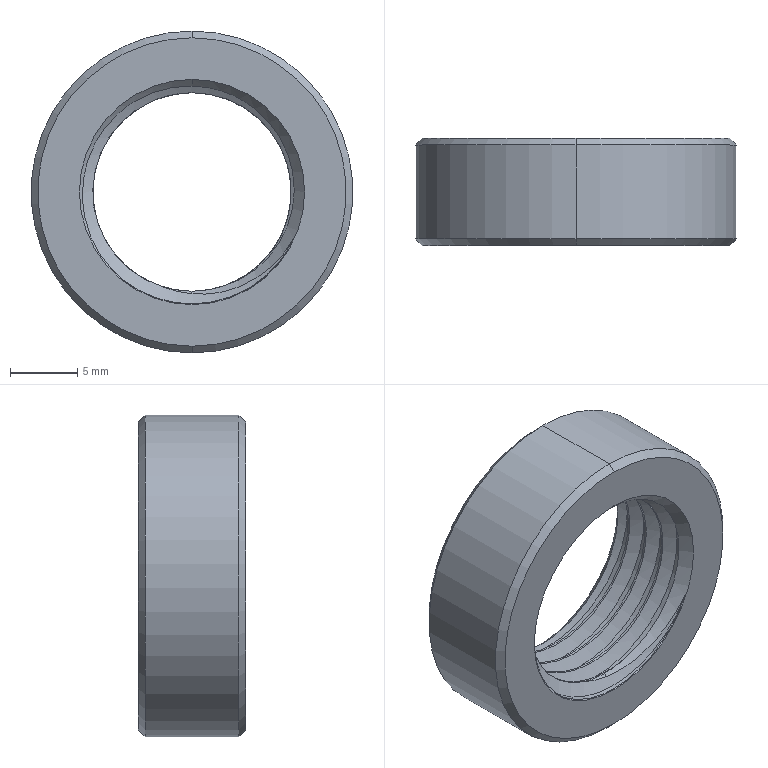Part | SolidWorks | features Chamfer 2, Extrusion 1, Helix 1, SweepCut 1 | 1 solid | 25 faces | box 24 x 8 x 24 mm | volume 1989 mm3 | cone 10 | cylinder 10 | spline 3 | plane 2 | commonest cylinder face diameters 14.8 x8 24 x2